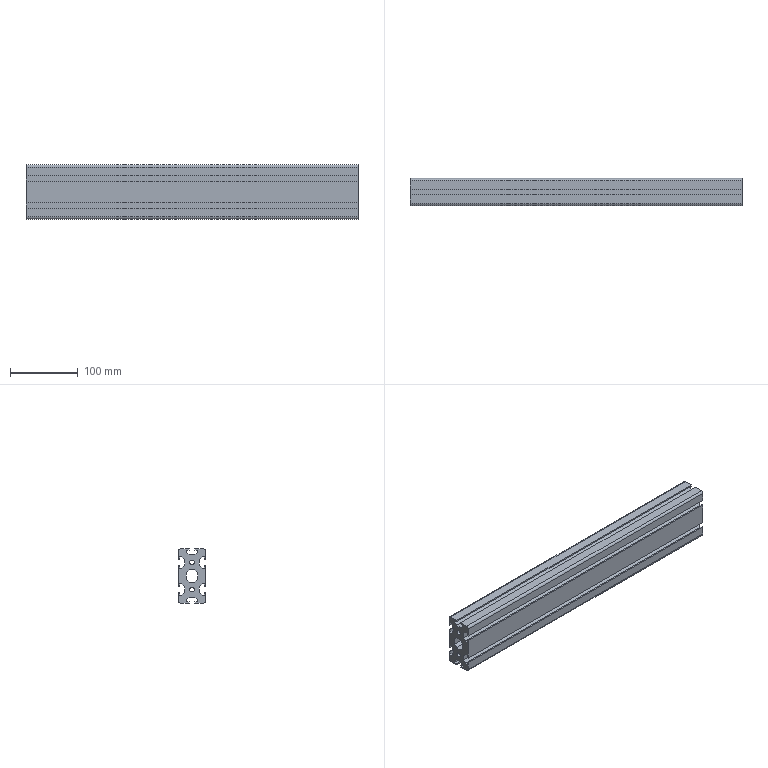Part | NX | 1 solid | 82 faces | box 490 x 40 x 80 mm | volume 1062076 mm3 | plane 74 | cylinder 8 | commonest cylinder face diameters 6.78 x4 6.8 x4